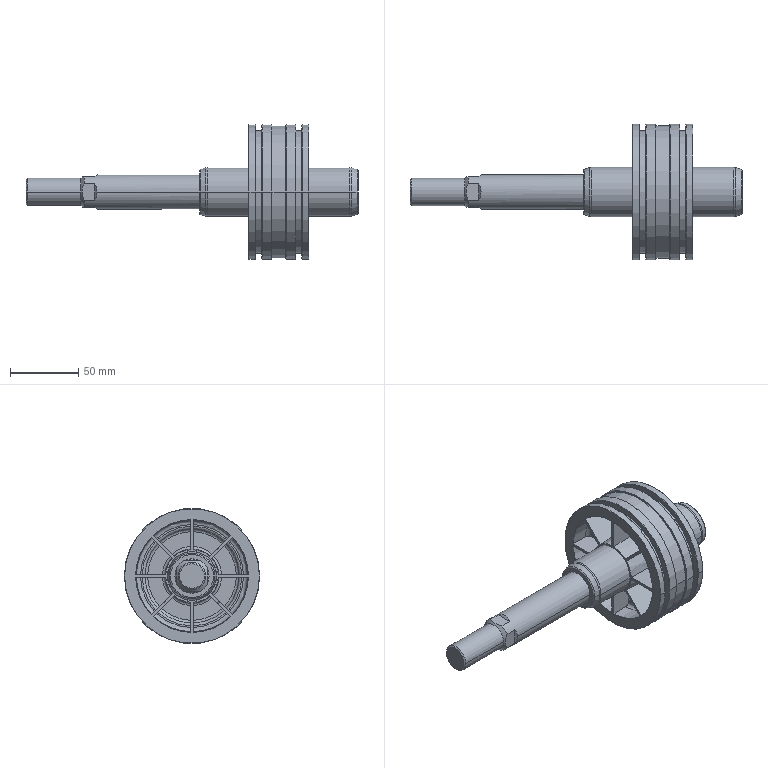Part | STEP file | 1 solid | 258 faces | box 243 x 99 x 99 mm | volume 277761 mm3 | plane 84 | torus 78 | cone 74 | cylinder 22 | commonest cylinder face diameters 99 x8 36 x4 90 x4 20 x2 25 x2 96.9 x2